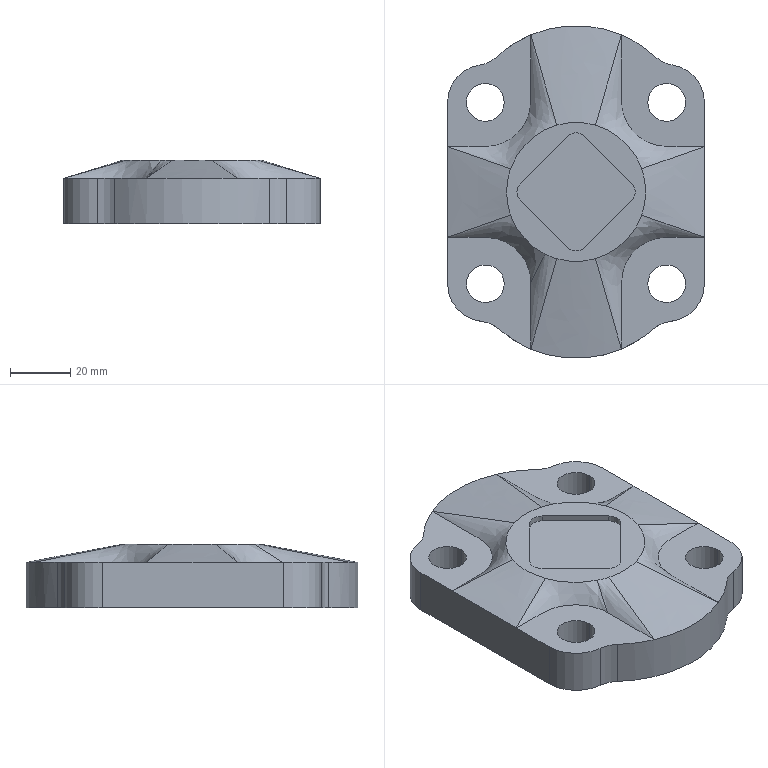Part | SolidWorks | features ICE 3, Fillet 2, Blend 1, Extrusion 1 | 1 solid | 51 faces | box 85 x 110 x 21 mm | volume 126964 mm3 | cylinder 27 | plane 15 | spline 9 | commonest cylinder face diameters 12.5 x8 8 x5 15 x4 20 x4 25 x4 77 x2